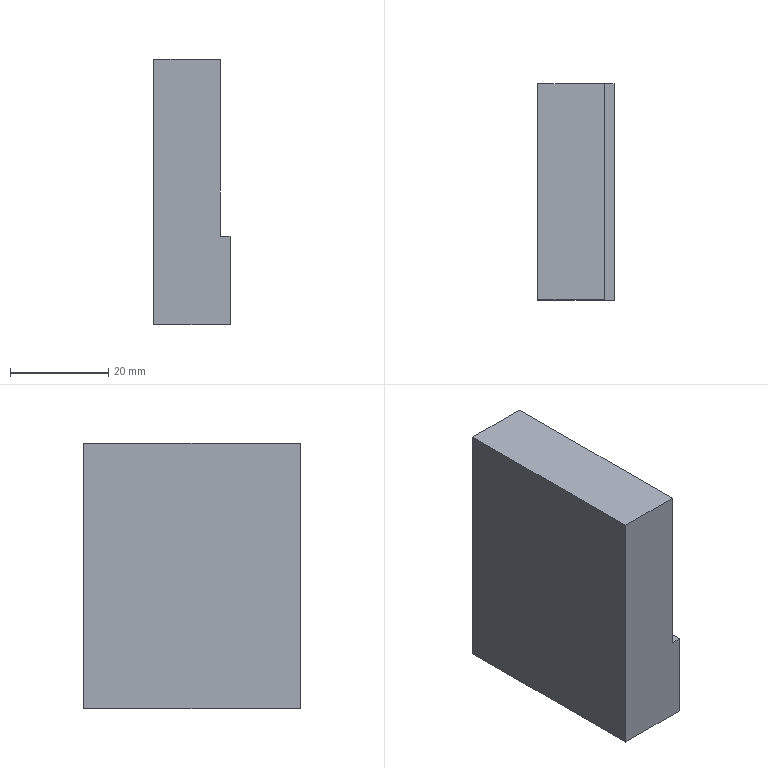Part | NX | features solid 2 | 1 solid | 8 faces | box 15.5 x 44 x 54 mm | volume 33660 mm3 | plane 8
STEP:
#1=CARTESIAN_POINT('',(-167.705,-135.535,126.));
#2=VERTEX_POINT('',#1);
#3=CARTESIAN_POINT('',(-167.705,-135.535,162.));
#4=VERTEX_POINT('',#3);
#5=CARTESIAN_POINT('',(-167.705,-135.535,108.));
#6=DIRECTION('',(0.,0.,1.));
#7=VECTOR('',#6,1000.);
#8=LINE('',#5,#7);
#9=EDGE_CURVE('',#2,#4,#8,.T.);
#10=ORIENTED_EDGE('',*,*,#9,.F.);
#11=CARTESIAN_POINT('',(-167.705,-91.535,126.));
#12=VERTEX_POINT('',#11);
#13=CARTESIAN_POINT('',(-167.705,-135.535,126.));
#14=DIRECTION('',(0.,1.,0.));
#15=VECTOR('',#14,1000.);
#16=LINE('',#13,#15);
#17=EDGE_CURVE('',#2,#12,#16,.T.);
#18=ORIENTED_EDGE('',*,*,#17,.T.);
#19=CARTESIAN_POINT('',(-167.705,-91.535,162.));
#20=VERTEX_POINT('',#19);
#21=CARTESIAN_POINT('',(-167.705,-91.535,108.));
#22=DIRECTION('',(0.,0.,1.));
#23=VECTOR('',#22,1000.);
#24=LINE('',#21,#23);
#25=EDGE_CURVE('',#12,#20,#24,.T.);
#26=ORIENTED_EDGE('',*,*,#25,.T.);
#27=CARTESIAN_POINT('',(-167.705,-135.535,162.));
#28=DIRECTION('',(0.,1.,0.));
#29=VECTOR('',#28,1000.);
#30=LINE('',#27,#29);
#31=EDGE_CURVE('',#4,#20,#30,.T.);
#32=ORIENTED_EDGE('',*,*,#31,.F.);
#33=EDGE_LOOP('',(#10,#18,#26,#32));
#34=FACE_BOUND('',#33,.T.);
#35=CARTESIAN_POINT('',(-167.705,-135.535,108.));
#36=DIRECTION('',(1.,0.,0.));
#37=DIRECTION('',(0.,1.,0.));
#38=AXIS2_PLACEMENT_3D('',#35,#36,#37);
#39=PLANE('',#38);
#40=ADVANCED_FACE('',(#34),#39,.T.);
#41=CARTESIAN_POINT('',(-181.205,-135.535,162.));
#42=VERTEX_POINT('',#41);
#43=CARTESIAN_POINT('',(-181.205,-91.535,162.));
#44=VERTEX_POINT('',#43);
#45=CARTESIAN_POINT('',(-181.205,-135.535,162.));
#46=DIRECTION('',(0.,1.,0.));
#47=VECTOR('',#46,1000.);
#48=LINE('',#45,#47);
#49=EDGE_CURVE('',#42,#44,#48,.T.);
#50=ORIENTED_EDGE('',*,*,#49,.F.);
#51=CARTESIAN_POINT('',(-167.705,-135.535,162.));
#52=DIRECTION('',(-1.,0.,0.));
#53=VECTOR('',#52,1000.);
#54=LINE('',#51,#53);
#55=EDGE_CURVE('',#4,#42,#54,.T.);
#56=ORIENTED_EDGE('',*,*,#55,.F.);
#57=ORIENTED_EDGE('',*,*,#31,.T.);
#58=CARTESIAN_POINT('',(-167.705,-91.535,162.));
#59=DIRECTION('',(-1.,0.,0.));
#60=VECTOR('',#59,1000.);
#61=LINE('',#58,#60);
#62=EDGE_CURVE('',#20,#44,#61,.T.);
#63=ORIENTED_EDGE('',*,*,#62,.T.);
#64=EDGE_LOOP('',(#50,#56,#57,#63));
#65=FACE_BOUND('',#64,.T.);
#66=CARTESIAN_POINT('',(-167.705,-135.535,162.));
#67=DIRECTION('',(0.,0.,1.));
#68=DIRECTION('',(1.,0.,0.));
#69=AXIS2_PLACEMENT_3D('',#66,#67,#68);
#70=PLANE('',#69);
#71=ADVANCED_FACE('',(#65),#70,.T.);
#72=CARTESIAN_POINT('',(-181.205,-135.535,108.));
#73=VERTEX_POINT('',#72);
#74=CARTESIAN_POINT('',(-181.205,-135.535,108.));
#75=DIRECTION('',(0.,0.,1.));
#76=VECTOR('',#75,1000.);
#77=LINE('',#74,#76);
#78=EDGE_CURVE('',#73,#42,#77,.T.);
#79=ORIENTED_EDGE('',*,*,#78,.F.);
#80=CARTESIAN_POINT('',(-165.705,-135.535,108.));
#81=VERTEX_POINT('',#80);
#82=CARTESIAN_POINT('',(-167.705,-135.535,108.));
#83=DIRECTION('',(-1.,0.,0.));
#84=VECTOR('',#83,1000.);
#85=LINE('',#82,#84);
#86=EDGE_CURVE('',#81,#73,#85,.T.);
#87=ORIENTED_EDGE('',*,*,#86,.F.);
#88=CARTESIAN_POINT('',(-165.705,-135.535,126.));
#89=VERTEX_POINT('',#88);
#90=CARTESIAN_POINT('',(-165.705,-135.535,108.));
#91=DIRECTION('',(0.,0.,1.));
#92=VECTOR('',#91,1000.);
#93=LINE('',#90,#92);
#94=EDGE_CURVE('',#81,#89,#93,.T.);
#95=ORIENTED_EDGE('',*,*,#94,.T.);
#96=CARTESIAN_POINT('',(-167.705,-135.535,126.));
#97=DIRECTION('',(1.,0.,0.));
#98=VECTOR('',#97,1000.);
#99=LINE('',#96,#98);
#100=EDGE_CURVE('',#89,#2,#99,.F.);
#101=ORIENTED_EDGE('',*,*,#100,.T.);
#102=ORIENTED_EDGE('',*,*,#9,.T.);
#103=ORIENTED_EDGE('',*,*,#55,.T.);
#104=EDGE_LOOP('',(#79,#87,#95,#101,#102,#103));
#105=FACE_BOUND('',#104,.T.);
#106=CARTESIAN_POINT('',(-167.705,-135.535,108.));
#107=DIRECTION('',(0.,-1.,0.));
#108=DIRECTION('',(0.,0.,-1.));
#109=AXIS2_PLACEMENT_3D('',#106,#107,#108);
#110=PLANE('',#109);
#111=ADVANCED_FACE('',(#105),#110,.T.);
#112=CARTESIAN_POINT('',(-181.205,-91.535,108.));
#113=VERTEX_POINT('',#112);
#114=CARTESIAN_POINT('',(-181.205,-135.535,108.));
#115=DIRECTION('',(0.,1.,0.));
#116=VECTOR('',#115,1000.);
#117=LINE('',#114,#116);
#118=EDGE_CURVE('',#73,#113,#117,.T.);
#119=ORIENTED_EDGE('',*,*,#118,.T.);
#120=CARTESIAN_POINT('',(-165.705,-91.535,108.));
#121=VERTEX_POINT('',#120);
#122=CARTESIAN_POINT('',(-167.705,-91.535,108.));
#123=DIRECTION('',(-1.,0.,0.));
#124=VECTOR('',#123,1000.);
#125=LINE('',#122,#124);
#126=EDGE_CURVE('',#121,#113,#125,.T.);
#127=ORIENTED_EDGE('',*,*,#126,.F.);
#128=CARTESIAN_POINT('',(-165.705,-135.535,108.));
#129=DIRECTION('',(0.,1.,0.));
#130=VECTOR('',#129,1000.);
#131=LINE('',#128,#130);
#132=EDGE_CURVE('',#81,#121,#131,.T.);
#133=ORIENTED_EDGE('',*,*,#132,.F.);
#134=ORIENTED_EDGE('',*,*,#86,.T.);
#135=EDGE_LOOP('',(#119,#127,#133,#134));
#136=FACE_BOUND('',#135,.T.);
#137=CARTESIAN_POINT('',(-167.705,-135.535,108.));
#138=DIRECTION('',(0.,0.,1.));
#139=DIRECTION('',(1.,0.,0.));
#140=AXIS2_PLACEMENT_3D('',#137,#138,#139);
#141=PLANE('',#140);
#142=ADVANCED_FACE('',(#136),#141,.F.);
#143=CARTESIAN_POINT('',(-181.205,-91.535,108.));
#144=DIRECTION('',(0.,0.,1.));
#145=VECTOR('',#144,1000.);
#146=LINE('',#143,#145);
#147=EDGE_CURVE('',#113,#44,#146,.T.);
#148=ORIENTED_EDGE('',*,*,#147,.T.);
#149=ORIENTED_EDGE('',*,*,#62,.F.);
#150=ORIENTED_EDGE('',*,*,#25,.F.);
#151=CARTESIAN_POINT('',(-165.705,-91.535,126.));
#152=VERTEX_POINT('',#151);
#153=CARTESIAN_POINT('',(-167.705,-91.535,126.));
#154=DIRECTION('',(1.,0.,0.));
#155=VECTOR('',#154,1000.);
#156=LINE('',#153,#155);
#157=EDGE_CURVE('',#152,#12,#156,.F.);
#158=ORIENTED_EDGE('',*,*,#157,.F.);
#159=CARTESIAN_POINT('',(-165.705,-91.535,108.));
#160=DIRECTION('',(0.,0.,1.));
#161=VECTOR('',#160,1000.);
#162=LINE('',#159,#161);
#163=EDGE_CURVE('',#121,#152,#162,.T.);
#164=ORIENTED_EDGE('',*,*,#163,.F.);
#165=ORIENTED_EDGE('',*,*,#126,.T.);
#166=EDGE_LOOP('',(#148,#149,#150,#158,#164,#165));
#167=FACE_BOUND('',#166,.T.);
#168=CARTESIAN_POINT('',(-167.705,-91.535,108.));
#169=DIRECTION('',(0.,-1.,0.));
#170=DIRECTION('',(0.,0.,-1.));
#171=AXIS2_PLACEMENT_3D('',#168,#169,#170);
#172=PLANE('',#171);
#173=ADVANCED_FACE('',(#167),#172,.F.);
#174=ORIENTED_EDGE('',*,*,#49,.T.);
#175=ORIENTED_EDGE('',*,*,#147,.F.);
#176=ORIENTED_EDGE('',*,*,#118,.F.);
#177=ORIENTED_EDGE('',*,*,#78,.T.);
#178=EDGE_LOOP('',(#174,#175,#176,#177));
#179=FACE_BOUND('',#178,.T.);
#180=CARTESIAN_POINT('',(-181.205,-135.535,108.));
#181=DIRECTION('',(1.,0.,0.));
#182=DIRECTION('',(0.,1.,0.));
#183=AXIS2_PLACEMENT_3D('',#180,#181,#182);
#184=PLANE('',#183);
#185=ADVANCED_FACE('',(#179),#184,.F.);
#186=ORIENTED_EDGE('',*,*,#157,.T.);
#187=ORIENTED_EDGE('',*,*,#17,.F.);
#188=ORIENTED_EDGE('',*,*,#100,.F.);
#189=CARTESIAN_POINT('',(-165.705,-135.535,126.));
#190=DIRECTION('',(0.,1.,0.));
#191=VECTOR('',#190,1000.);
#192=LINE('',#189,#191);
#193=EDGE_CURVE('',#89,#152,#192,.T.);
#194=ORIENTED_EDGE('',*,*,#193,.T.);
#195=EDGE_LOOP('',(#186,#187,#188,#194));
#196=FACE_BOUND('',#195,.T.);
#197=CARTESIAN_POINT('',(-167.705,-135.535,126.));
#198=DIRECTION('',(0.,0.,-1.));
#199=DIRECTION('',(0.,1.,0.));
#200=AXIS2_PLACEMENT_3D('',#197,#198,#199);
#201=PLANE('',#200);
#202=ADVANCED_FACE('',(#196),#201,.F.);
#203=ORIENTED_EDGE('',*,*,#193,.F.);
#204=ORIENTED_EDGE('',*,*,#94,.F.);
#205=ORIENTED_EDGE('',*,*,#132,.T.);
#206=ORIENTED_EDGE('',*,*,#163,.T.);
#207=EDGE_LOOP('',(#203,#204,#205,#206));
#208=FACE_BOUND('',#207,.T.);
#209=CARTESIAN_POINT('',(-165.705,-135.535,108.));
#210=DIRECTION('',(1.,0.,0.));
#211=DIRECTION('',(0.,1.,0.));
#212=AXIS2_PLACEMENT_3D('',#209,#210,#211);
#213=PLANE('',#212);
#214=ADVANCED_FACE('',(#208),#213,.T.);
#215=CLOSED_SHELL('',(#40,#71,#111,#142,#173,#185,#202,#214));
#216=MANIFOLD_SOLID_BREP('',#215);
#217=(LENGTH_UNIT()NAMED_UNIT(*)SI_UNIT(.MILLI.,.METRE.));
#218=UNCERTAINTY_MEASURE_WITH_UNIT(LENGTH_MEASURE(0.00001),#217,'','');
#219=(NAMED_UNIT(*)PLANE_ANGLE_UNIT()SI_UNIT($,.RADIAN.));
#220=(NAMED_UNIT(*)SI_UNIT($,.STERADIAN.)SOLID_ANGLE_UNIT());
#221=(GEOMETRIC_REPRESENTATION_CONTEXT(3)GLOBAL_UNCERTAINTY_ASSIGNED_CONTEXT((#218))GLOBAL_UNIT_ASSIGNED_CONTEXT((#217,#219,#220))REPRESENTATION_CONTEXT('',''));
#222=ADVANCED_BREP_SHAPE_REPRESENTATION('',(#216),#221);